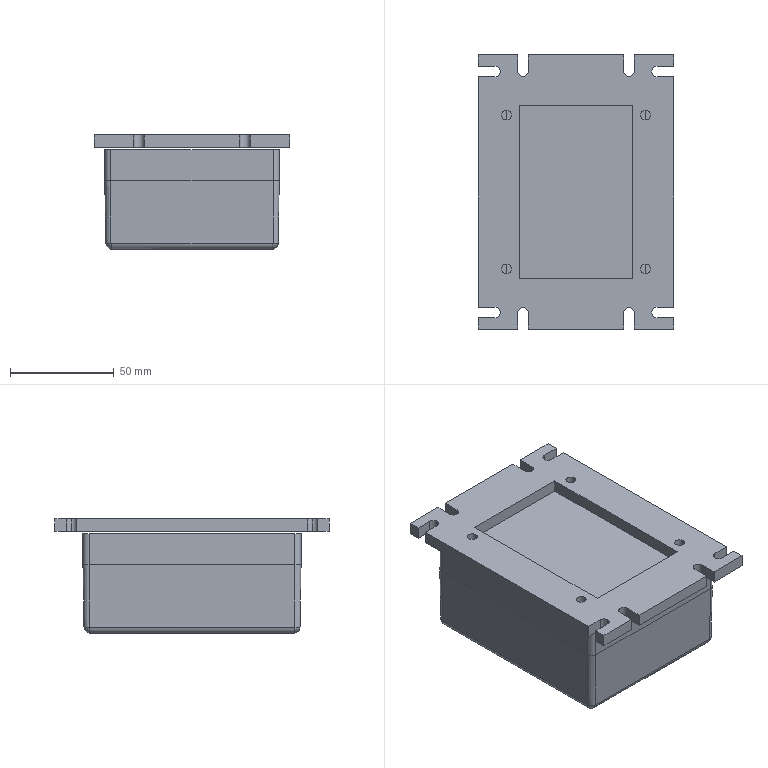Part | SolidWorks | features BaseBody 3 | 3 solids | 88 faces | box 94 x 132 x 55 mm | volume 461211 mm3 | plane 54 | cylinder 26 | spline 4 | cone 4 | commonest cylinder face diameters 5 x10 4.7 x8 6 x8